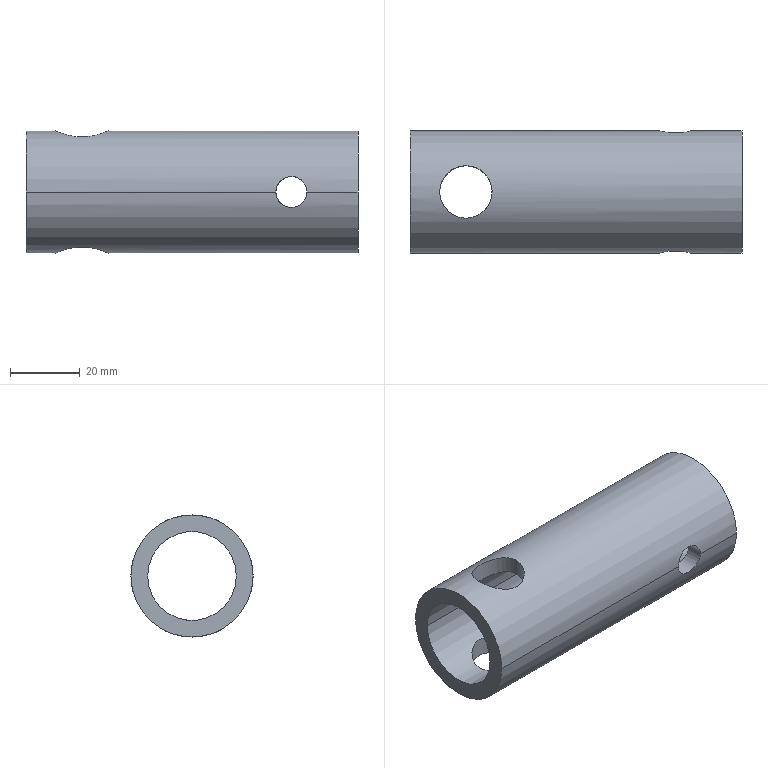Part | NX | features BREP 1 | 1 solid | 14 faces | box 94.996 x 34.925 x 34.925 mm | volume 40535 mm3 | cylinder 12 | plane 2 | commonest cylinder face diameters 8.89 x4 14.986 x4 25.4 x2 34.925 x2
STEP:
#1=CARTESIAN_POINT('',(-47.498,17.462,0.));
#2=VERTEX_POINT('',#1);
#3=CARTESIAN_POINT('',(-47.498,-17.462,0.));
#4=VERTEX_POINT('',#3);
#5=CARTESIAN_POINT('',(-47.498,0.,0.));
#6=DIRECTION('',(1.,0.,0.));
#7=DIRECTION('',(0.,1.,0.));
#8=AXIS2_PLACEMENT_3D('',#5,#6,#7);
#9=CIRCLE('',#8,17.462);
#10=EDGE_CURVE('',#2,#4,#9,.T.);
#11=ORIENTED_EDGE('',*,*,#10,.F.);
#12=CARTESIAN_POINT('',(-47.498,0.,0.));
#13=DIRECTION('',(1.,0.,0.));
#14=DIRECTION('',(0.,-1.,0.));
#15=AXIS2_PLACEMENT_3D('',#12,#13,#14);
#16=CIRCLE('',#15,17.462);
#17=EDGE_CURVE('',#4,#2,#16,.T.);
#18=ORIENTED_EDGE('',*,*,#17,.F.);
#19=EDGE_LOOP('',(#11,#18));
#20=FACE_BOUND('',#19,.T.);
#21=CARTESIAN_POINT('',(-47.498,12.7,0.));
#22=VERTEX_POINT('',#21);
#23=CARTESIAN_POINT('',(-47.498,-12.7,0.));
#24=VERTEX_POINT('',#23);
#25=CARTESIAN_POINT('',(-47.498,0.,0.));
#26=DIRECTION('',(-1.,0.,0.));
#27=DIRECTION('',(0.,1.,0.));
#28=AXIS2_PLACEMENT_3D('',#25,#26,#27);
#29=CIRCLE('',#28,12.7);
#30=EDGE_CURVE('',#22,#24,#29,.T.);
#31=ORIENTED_EDGE('',*,*,#30,.F.);
#32=CARTESIAN_POINT('',(-47.498,0.,0.));
#33=DIRECTION('',(-1.,0.,0.));
#34=DIRECTION('',(0.,-1.,0.));
#35=AXIS2_PLACEMENT_3D('',#32,#33,#34);
#36=CIRCLE('',#35,12.7);
#37=EDGE_CURVE('',#24,#22,#36,.T.);
#38=ORIENTED_EDGE('',*,*,#37,.F.);
#39=EDGE_LOOP('',(#31,#38));
#40=FACE_BOUND('',#39,.T.);
#41=CARTESIAN_POINT('',(-47.498,0.,0.));
#42=DIRECTION('',(1.,0.,0.));
#43=DIRECTION('',(0.,1.,0.));
#44=AXIS2_PLACEMENT_3D('',#41,#42,#43);
#45=PLANE('',#44);
#46=ADVANCED_FACE('',(#20,#40),#45,.F.);
#47=CARTESIAN_POINT('',(24.003,-17.462,0.));
#48=VERTEX_POINT('',#47);
#49=CARTESIAN_POINT('',(-47.498,-17.462,0.));
#50=DIRECTION('',(1.,0.,0.));
#51=VECTOR('',#50,1000.);
#52=LINE('',#49,#51);
#53=EDGE_CURVE('',#48,#4,#52,.F.);
#54=ORIENTED_EDGE('',*,*,#53,.T.);
#55=ORIENTED_EDGE('',*,*,#17,.T.);
#56=CARTESIAN_POINT('',(24.003,17.462,0.));
#57=VERTEX_POINT('',#56);
#58=CARTESIAN_POINT('',(-47.498,17.462,0.));
#59=DIRECTION('',(1.,0.,0.));
#60=VECTOR('',#59,1000.);
#61=LINE('',#58,#60);
#62=EDGE_CURVE('',#57,#2,#61,.F.);
#63=ORIENTED_EDGE('',*,*,#62,.F.);
#64=CARTESIAN_POINT('',(32.893,17.462,0.));
#65=VERTEX_POINT('',#64);
#66=CARTESIAN_POINT('',(24.003,17.462,0.));
#67=CARTESIAN_POINT('',(24.003,17.462,-1.164));
#68=CARTESIAN_POINT('',(24.94,17.187,-3.444));
#69=CARTESIAN_POINT('',(28.412,16.74,-4.935));
#70=CARTESIAN_POINT('',(31.928,17.178,-3.487));
#71=CARTESIAN_POINT('',(32.893,17.462,-1.178));
#72=CARTESIAN_POINT('',(32.893,17.462,0.));
#73=B_SPLINE_CURVE_WITH_KNOTS('',3,(#66,#67,#68,#69,#70,#71,#72),.UNSPECIFIED.,.F.,.F.,(4,1,1,1,4),(0.,0.25,0.5,0.75,1.),.UNSPECIFIED.);
#74=EDGE_CURVE('',#57,#65,#73,.T.);
#75=ORIENTED_EDGE('',*,*,#74,.T.);
#76=CARTESIAN_POINT('',(47.498,17.462,0.));
#77=VERTEX_POINT('',#76);
#78=CARTESIAN_POINT('',(32.893,17.462,0.));
#79=DIRECTION('',(1.,0.,0.));
#80=VECTOR('',#79,1000.);
#81=LINE('',#78,#80);
#82=EDGE_CURVE('',#65,#77,#81,.T.);
#83=ORIENTED_EDGE('',*,*,#82,.T.);
#84=CARTESIAN_POINT('',(47.498,-17.462,0.));
#85=VERTEX_POINT('',#84);
#86=CARTESIAN_POINT('',(47.498,0.,0.));
#87=DIRECTION('',(1.,0.,0.));
#88=DIRECTION('',(0.,-1.,0.));
#89=AXIS2_PLACEMENT_3D('',#86,#87,#88);
#90=CIRCLE('',#89,17.462);
#91=EDGE_CURVE('',#85,#77,#90,.T.);
#92=ORIENTED_EDGE('',*,*,#91,.F.);
#93=CARTESIAN_POINT('',(32.893,-17.462,0.));
#94=VERTEX_POINT('',#93);
#95=CARTESIAN_POINT('',(32.893,-17.462,0.));
#96=DIRECTION('',(1.,0.,0.));
#97=VECTOR('',#96,1000.);
#98=LINE('',#95,#97);
#99=EDGE_CURVE('',#94,#85,#98,.T.);
#100=ORIENTED_EDGE('',*,*,#99,.F.);
#101=CARTESIAN_POINT('',(32.893,-17.462,0.));
#102=CARTESIAN_POINT('',(32.893,-17.462,-1.177));
#103=CARTESIAN_POINT('',(31.929,-17.178,-3.484));
#104=CARTESIAN_POINT('',(28.419,-16.74,-4.934));
#105=CARTESIAN_POINT('',(24.943,-17.185,-3.449));
#106=CARTESIAN_POINT('',(24.003,-17.462,-1.165));
#107=CARTESIAN_POINT('',(24.003,-17.462,0.));
#108=B_SPLINE_CURVE_WITH_KNOTS('',3,(#101,#102,#103,#104,#105,#106,#107),.UNSPECIFIED.,.F.,.F.,(4,1,1,1,4),(0.,0.25,0.5,0.75,1.),.UNSPECIFIED.);
#109=EDGE_CURVE('',#94,#48,#108,.T.);
#110=ORIENTED_EDGE('',*,*,#109,.T.);
#111=EDGE_LOOP('',(#54,#55,#63,#75,#83,#92,#100,#110));
#112=FACE_BOUND('',#111,.T.);
#113=CARTESIAN_POINT('',(-38.989,0.,-17.462));
#114=VERTEX_POINT('',#113);
#115=CARTESIAN_POINT('',(-24.003,0.,-17.462));
#116=VERTEX_POINT('',#115);
#117=CARTESIAN_POINT('',(-38.989,0.,-17.462));
#118=CARTESIAN_POINT('',(-38.989,-2.022,-17.462));
#119=CARTESIAN_POINT('',(-37.692,-4.958,-16.852));
#120=CARTESIAN_POINT('',(-34.426,-7.1,-15.966));
#121=CARTESIAN_POINT('',(-31.48,-7.694,-15.675));
#122=CARTESIAN_POINT('',(-28.528,-7.083,-15.973));
#123=CARTESIAN_POINT('',(-25.304,-4.95,-16.853));
#124=CARTESIAN_POINT('',(-24.003,-2.022,-17.462));
#125=CARTESIAN_POINT('',(-24.003,0.,-17.462));
#126=B_SPLINE_CURVE_WITH_KNOTS('',3,(#117,#118,#119,#120,#121,#122,#123,#124,#125),.UNSPECIFIED.,.F.,.F.,(4,1,1,1,1,1,4),(0.,0.25,0.375,0.5,0.625,0.75,1.),.UNSPECIFIED.);
#127=EDGE_CURVE('',#114,#116,#126,.T.);
#128=ORIENTED_EDGE('',*,*,#127,.T.);
#129=CARTESIAN_POINT('',(-24.003,0.,-17.462));
#130=CARTESIAN_POINT('',(-24.003,2.019,-17.462));
#131=CARTESIAN_POINT('',(-25.295,4.952,-16.853));
#132=CARTESIAN_POINT('',(-28.564,7.1,-15.966));
#133=CARTESIAN_POINT('',(-31.512,7.694,-15.675));
#134=CARTESIAN_POINT('',(-34.465,7.083,-15.974));
#135=CARTESIAN_POINT('',(-37.693,4.945,-16.855));
#136=CARTESIAN_POINT('',(-38.989,2.019,-17.462));
#137=CARTESIAN_POINT('',(-38.989,0.,-17.462));
#138=B_SPLINE_CURVE_WITH_KNOTS('',3,(#129,#130,#131,#132,#133,#134,#135,#136,#137),.UNSPECIFIED.,.F.,.F.,(4,1,1,1,1,1,4),(0.,0.25,0.375,0.5,0.625,0.75,1.),.UNSPECIFIED.);
#139=EDGE_CURVE('',#116,#114,#138,.T.);
#140=ORIENTED_EDGE('',*,*,#139,.T.);
#141=EDGE_LOOP('',(#128,#140));
#142=FACE_BOUND('',#141,.T.);
#143=CARTESIAN_POINT('',(-47.498,0.,0.));
#144=DIRECTION('',(1.,0.,0.));
#145=DIRECTION('',(0.,-1.,0.));
#146=AXIS2_PLACEMENT_3D('',#143,#144,#145);
#147=CYLINDRICAL_SURFACE('',#146,17.462);
#148=ADVANCED_FACE('',(#112,#142),#147,.T.);
#149=CARTESIAN_POINT('',(32.893,-12.7,0.));
#150=VERTEX_POINT('',#149);
#151=CARTESIAN_POINT('',(32.893,-12.7,0.));
#152=DIRECTION('',(0.,-1.,0.));
#153=VECTOR('',#152,1000.);
#154=LINE('',#151,#153);
#155=EDGE_CURVE('',#94,#150,#154,.F.);
#156=ORIENTED_EDGE('',*,*,#155,.T.);
#157=CARTESIAN_POINT('',(24.003,-12.7,0.));
#158=VERTEX_POINT('',#157);
#159=CARTESIAN_POINT('',(32.893,-12.7,0.));
#160=CARTESIAN_POINT('',(32.893,-12.7,-0.278));
#161=CARTESIAN_POINT('',(32.848,-12.683,-0.8361));
#162=CARTESIAN_POINT('',(32.607,-12.602,-1.608));
#163=CARTESIAN_POINT('',(32.389,-12.532,-2.073));
#164=CARTESIAN_POINT('',(32.124,-12.451,-2.511));
#165=CARTESIAN_POINT('',(31.944,-12.399,-2.753));
#166=CARTESIAN_POINT('',(31.605,-12.306,-3.15));
#167=CARTESIAN_POINT('',(31.156,-12.2,-3.532));
#168=CARTESIAN_POINT('',(30.958,-12.157,-3.675));
#169=CARTESIAN_POINT('',(30.5,-12.07,-3.953));
#170=CARTESIAN_POINT('',(30.042,-11.999,-4.162));
#171=CARTESIAN_POINT('',(29.303,-11.916,-4.396));
#172=CARTESIAN_POINT('',(28.425,-11.886,-4.472));
#173=CARTESIAN_POINT('',(27.547,-11.919,-4.387));
#174=CARTESIAN_POINT('',(26.807,-12.005,-4.144));
#175=CARTESIAN_POINT('',(26.358,-12.077,-3.934));
#176=CARTESIAN_POINT('',(25.9,-12.165,-3.648));
#177=CARTESIAN_POINT('',(25.721,-12.204,-3.518));
#178=CARTESIAN_POINT('',(25.263,-12.313,-3.122));
#179=CARTESIAN_POINT('',(24.94,-12.403,-2.736));
#180=CARTESIAN_POINT('',(24.756,-12.456,-2.488));
#181=CARTESIAN_POINT('',(24.498,-12.535,-2.055));
#182=CARTESIAN_POINT('',(24.283,-12.604,-1.592));
#183=CARTESIAN_POINT('',(24.048,-12.683,-0.8289));
#184=CARTESIAN_POINT('',(24.003,-12.7,-0.2756));
#185=CARTESIAN_POINT('',(24.003,-12.7,0.));
#186=B_SPLINE_CURVE_WITH_KNOTS('',3,(#159,#160,#161,#162,#163,#164,#165,#166,#167,#168,#169,#170,#171,#172,#173,#174,#175,#176,#177,#178,#179,#180,#181,#182,#183,#184,#185),.UNSPECIFIED.,.F.,.F.,(4,1,1,1,1,1,1,1,1,1,1,1,1,1,1,1,1,1,1,1,1,1,1,1,4),(0.,0.0625,0.125,0.1562,0.1875,0.2188,0.25,0.2812,0.3125,0.3438,0.375,0.4375,0.5,0.5625,0.625,0.6562,0.6875,0.7188,0.75,0.7812,0.8125,0.8438,0.875,0.9375,1.),.UNSPECIFIED.);
#187=EDGE_CURVE('',#158,#150,#186,.F.);
#188=ORIENTED_EDGE('',*,*,#187,.F.);
#189=CARTESIAN_POINT('',(24.003,-12.7,0.));
#190=DIRECTION('',(0.,-1.,0.));
#191=VECTOR('',#190,1000.);
#192=LINE('',#189,#191);
#193=EDGE_CURVE('',#48,#158,#192,.F.);
#194=ORIENTED_EDGE('',*,*,#193,.F.);
#195=ORIENTED_EDGE('',*,*,#109,.F.);
#196=EDGE_LOOP('',(#156,#188,#194,#195));
#197=FACE_BOUND('',#196,.T.);
#198=CARTESIAN_POINT('',(28.448,22.86,0.));
#199=DIRECTION('',(0.,1.,0.));
#200=DIRECTION('',(1.,0.,0.));
#201=AXIS2_PLACEMENT_3D('',#198,#199,#200);
#202=CYLINDRICAL_SURFACE('',#201,4.445);
#203=ADVANCED_FACE('',(#197),#202,.F.);
#204=CARTESIAN_POINT('',(24.003,12.7,0.));
#205=VERTEX_POINT('',#204);
#206=CARTESIAN_POINT('',(24.003,17.462,0.));
#207=DIRECTION('',(0.,-1.,0.));
#208=VECTOR('',#207,1000.);
#209=LINE('',#206,#208);
#210=EDGE_CURVE('',#57,#205,#209,.T.);
#211=ORIENTED_EDGE('',*,*,#210,.T.);
#212=CARTESIAN_POINT('',(32.893,12.7,0.));
#213=VERTEX_POINT('',#212);
#214=CARTESIAN_POINT('',(24.003,12.7,0.));
#215=CARTESIAN_POINT('',(24.003,12.7,-0.2753));
#216=CARTESIAN_POINT('',(24.048,12.683,-0.828));
#217=CARTESIAN_POINT('',(24.283,12.604,-1.59));
#218=CARTESIAN_POINT('',(24.497,12.535,-2.053));
#219=CARTESIAN_POINT('',(24.755,12.456,-2.485));
#220=CARTESIAN_POINT('',(24.938,12.403,-2.734));
#221=CARTESIAN_POINT('',(25.259,12.314,-3.118));
#222=CARTESIAN_POINT('',(25.719,12.205,-3.516));
#223=CARTESIAN_POINT('',(25.894,12.166,-3.645));
#224=CARTESIAN_POINT('',(26.353,12.077,-3.931));
#225=CARTESIAN_POINT('',(26.801,12.006,-4.141));
#226=CARTESIAN_POINT('',(27.541,11.919,-4.386));
#227=CARTESIAN_POINT('',(28.42,11.886,-4.472));
#228=CARTESIAN_POINT('',(29.299,11.915,-4.397));
#229=CARTESIAN_POINT('',(30.038,11.998,-4.164));
#230=CARTESIAN_POINT('',(30.497,12.07,-3.955));
#231=CARTESIAN_POINT('',(30.955,12.156,-3.677));
#232=CARTESIAN_POINT('',(31.154,12.2,-3.533));
#233=CARTESIAN_POINT('',(31.603,12.305,-3.152));
#234=CARTESIAN_POINT('',(31.943,12.399,-2.754));
#235=CARTESIAN_POINT('',(32.123,12.451,-2.513));
#236=CARTESIAN_POINT('',(32.389,12.532,-2.074));
#237=CARTESIAN_POINT('',(32.606,12.602,-1.61));
#238=CARTESIAN_POINT('',(32.848,12.683,-0.8367));
#239=CARTESIAN_POINT('',(32.893,12.7,-0.2782));
#240=CARTESIAN_POINT('',(32.893,12.7,0.));
#241=B_SPLINE_CURVE_WITH_KNOTS('',3,(#214,#215,#216,#217,#218,#219,#220,#221,#222,#223,#224,#225,#226,#227,#228,#229,#230,#231,#232,#233,#234,#235,#236,#237,#238,#239,#240),.UNSPECIFIED.,.F.,.F.,(4,1,1,1,1,1,1,1,1,1,1,1,1,1,1,1,1,1,1,1,1,1,1,1,4),(0.,0.0625,0.125,0.1562,0.1875,0.2188,0.25,0.2812,0.3125,0.3438,0.375,0.4375,0.5,0.5625,0.625,0.6562,0.6875,0.7188,0.75,0.7812,0.8125,0.8438,0.875,0.9375,1.),.UNSPECIFIED.);
#242=EDGE_CURVE('',#213,#205,#241,.F.);
#243=ORIENTED_EDGE('',*,*,#242,.F.);
#244=CARTESIAN_POINT('',(32.893,17.462,0.));
#245=DIRECTION('',(0.,-1.,0.));
#246=VECTOR('',#245,1000.);
#247=LINE('',#244,#246);
#248=EDGE_CURVE('',#65,#213,#247,.T.);
#249=ORIENTED_EDGE('',*,*,#248,.F.);
#250=ORIENTED_EDGE('',*,*,#74,.F.);
#251=EDGE_LOOP('',(#211,#243,#249,#250));
#252=FACE_BOUND('',#251,.T.);
#253=CARTESIAN_POINT('',(28.448,22.86,0.));
#254=DIRECTION('',(0.,1.,0.));
#255=DIRECTION('',(1.,0.,0.));
#256=AXIS2_PLACEMENT_3D('',#253,#254,#255);
#257=CYLINDRICAL_SURFACE('',#256,4.445);
#258=ADVANCED_FACE('',(#252),#257,.F.);
#259=ORIENTED_EDGE('',*,*,#248,.T.);
#260=CARTESIAN_POINT('',(32.893,12.7,0.));
#261=CARTESIAN_POINT('',(32.893,12.7,0.2756));
#262=CARTESIAN_POINT('',(32.848,12.683,0.8289));
#263=CARTESIAN_POINT('',(32.613,12.604,1.592));
#264=CARTESIAN_POINT('',(32.398,12.535,2.055));
#265=CARTESIAN_POINT('',(32.14,12.456,2.488));
#266=CARTESIAN_POINT('',(31.956,12.403,2.736));
#267=CARTESIAN_POINT('',(31.633,12.313,3.122));
#268=CARTESIAN_POINT('',(31.174,12.204,3.518));
#269=CARTESIAN_POINT('',(30.997,12.165,3.648));
#270=CARTESIAN_POINT('',(30.537,12.077,3.934));
#271=CARTESIAN_POINT('',(30.089,12.006,4.144));
#272=CARTESIAN_POINT('',(29.349,11.919,4.387));
#273=CARTESIAN_POINT('',(28.471,11.886,4.472));
#274=CARTESIAN_POINT('',(27.593,11.916,4.396));
#275=CARTESIAN_POINT('',(26.855,11.999,4.163));
#276=CARTESIAN_POINT('',(26.396,12.07,3.953));
#277=CARTESIAN_POINT('',(25.938,12.157,3.675));
#278=CARTESIAN_POINT('',(25.74,12.2,3.532));
#279=CARTESIAN_POINT('',(25.291,12.306,3.15));
#280=CARTESIAN_POINT('',(24.952,12.399,2.753));
#281=CARTESIAN_POINT('',(24.772,12.451,2.511));
#282=CARTESIAN_POINT('',(24.507,12.532,2.073));
#283=CARTESIAN_POINT('',(24.289,12.602,1.608));
#284=CARTESIAN_POINT('',(24.048,12.683,0.8362));
#285=CARTESIAN_POINT('',(24.003,12.7,0.2781));
#286=CARTESIAN_POINT('',(24.003,12.7,0.));
#287=B_SPLINE_CURVE_WITH_KNOTS('',3,(#260,#261,#262,#263,#264,#265,#266,#267,#268,#269,#270,#271,#272,#273,#274,#275,#276,#277,#278,#279,#280,#281,#282,#283,#284,#285,#286),.UNSPECIFIED.,.F.,.F.,(4,1,1,1,1,1,1,1,1,1,1,1,1,1,1,1,1,1,1,1,1,1,1,1,4),(0.,0.0625,0.125,0.1562,0.1875,0.2188,0.25,0.2812,0.3125,0.3438,0.375,0.4375,0.5,0.5625,0.625,0.6562,0.6875,0.7188,0.75,0.7812,0.8125,0.8438,0.875,0.9375,1.),.UNSPECIFIED.);
#288=EDGE_CURVE('',#205,#213,#287,.F.);
#289=ORIENTED_EDGE('',*,*,#288,.F.);
#290=ORIENTED_EDGE('',*,*,#210,.F.);
#291=CARTESIAN_POINT('',(24.003,17.462,0.));
#292=CARTESIAN_POINT('',(24.003,17.462,0.2769));
#293=CARTESIAN_POINT('',(24.048,17.45,0.833));
#294=CARTESIAN_POINT('',(24.289,17.392,1.606));
#295=CARTESIAN_POINT('',(24.504,17.341,2.069));
#296=CARTESIAN_POINT('',(24.773,17.282,2.512));
#297=CARTESIAN_POINT('',(24.945,17.246,2.744));
#298=CARTESIAN_POINT('',(25.299,17.177,3.157));
#299=CARTESIAN_POINT('',(25.727,17.105,3.521));
#300=CARTESIAN_POINT('',(25.947,17.07,3.682));
#301=CARTESIAN_POINT('',(26.401,17.009,3.955));
#302=CARTESIAN_POINT('',(26.856,16.959,4.164));
#303=CARTESIAN_POINT('',(27.64,16.899,4.406));
#304=CARTESIAN_POINT('',(28.472,16.881,4.467));
#305=CARTESIAN_POINT('',(29.299,16.901,4.398));
#306=CARTESIAN_POINT('',(30.086,16.963,4.146));
#307=CARTESIAN_POINT('',(30.534,17.014,3.935));
#308=CARTESIAN_POINT('',(30.988,17.076,3.655));
#309=CARTESIAN_POINT('',(31.185,17.107,3.51));
#310=CARTESIAN_POINT('',(31.626,17.182,3.129));
#311=CARTESIAN_POINT('',(31.962,17.248,2.73));
#312=CARTESIAN_POINT('',(32.138,17.285,2.49));
#313=CARTESIAN_POINT('',(32.4,17.343,2.052));
#314=CARTESIAN_POINT('',(32.613,17.393,1.59));
#315=CARTESIAN_POINT('',(32.849,17.45,0.8261));
#316=CARTESIAN_POINT('',(32.893,17.462,0.2746));
#317=CARTESIAN_POINT('',(32.893,17.462,0.));
#318=B_SPLINE_CURVE_WITH_KNOTS('',3,(#291,#292,#293,#294,#295,#296,#297,#298,#299,#300,#301,#302,#303,#304,#305,#306,#307,#308,#309,#310,#311,#312,#313,#314,#315,#316,#317),.UNSPECIFIED.,.F.,.F.,(4,1,1,1,1,1,1,1,1,1,1,1,1,1,1,1,1,1,1,1,1,1,1,1,4),(0.,0.0625,0.125,0.1562,0.1875,0.2188,0.25,0.2812,0.3125,0.3438,0.375,0.4375,0.5,0.5625,0.625,0.6562,0.6875,0.7188,0.75,0.7812,0.8125,0.8438,0.875,0.9375,1.),.UNSPECIFIED.);
#319=EDGE_CURVE('',#65,#57,#318,.F.);
#320=ORIENTED_EDGE('',*,*,#319,.F.);
#321=EDGE_LOOP('',(#259,#289,#290,#320));
#322=FACE_BOUND('',#321,.T.);
#323=CARTESIAN_POINT('',(28.448,22.86,0.));
#324=DIRECTION('',(0.,1.,0.));
#325=DIRECTION('',(1.,0.,0.));
#326=AXIS2_PLACEMENT_3D('',#323,#324,#325);
#327=CYLINDRICAL_SURFACE('',#326,4.445);
#328=ADVANCED_FACE('',(#322),#327,.F.);
#329=ORIENTED_EDGE('',*,*,#193,.T.);
#330=CARTESIAN_POINT('',(24.003,-12.7,0.));
#331=CARTESIAN_POINT('',(24.003,-12.7,0.2782));
#332=CARTESIAN_POINT('',(24.048,-12.683,0.8366));
#333=CARTESIAN_POINT('',(24.29,-12.602,1.61));
#334=CARTESIAN_POINT('',(24.507,-12.532,2.074));
#335=CARTESIAN_POINT('',(24.773,-12.451,2.513));
#336=CARTESIAN_POINT('',(24.953,-12.399,2.754));
#337=CARTESIAN_POINT('',(25.293,-12.305,3.152));
#338=CARTESIAN_POINT('',(25.742,-12.2,3.533));
#339=CARTESIAN_POINT('',(25.941,-12.156,3.677));
#340=CARTESIAN_POINT('',(26.399,-12.07,3.955));
#341=CARTESIAN_POINT('',(26.858,-11.998,4.164));
#342=CARTESIAN_POINT('',(27.597,-11.915,4.397));
#343=CARTESIAN_POINT('',(28.476,-11.886,4.472));
#344=CARTESIAN_POINT('',(29.355,-11.919,4.386));
#345=CARTESIAN_POINT('',(30.095,-12.006,4.141));
#346=CARTESIAN_POINT('',(30.543,-12.077,3.931));
#347=CARTESIAN_POINT('',(31.002,-12.166,3.645));
#348=CARTESIAN_POINT('',(31.177,-12.205,3.516));
#349=CARTESIAN_POINT('',(31.637,-12.314,3.118));
#350=CARTESIAN_POINT('',(31.958,-12.403,2.734));
#351=CARTESIAN_POINT('',(32.142,-12.456,2.485));
#352=CARTESIAN_POINT('',(32.399,-12.535,2.053));
#353=CARTESIAN_POINT('',(32.613,-12.604,1.59));
#354=CARTESIAN_POINT('',(32.848,-12.683,0.8281));
#355=CARTESIAN_POINT('',(32.893,-12.7,0.2753));
#356=CARTESIAN_POINT('',(32.893,-12.7,0.));
#357=B_SPLINE_CURVE_WITH_KNOTS('',3,(#330,#331,#332,#333,#334,#335,#336,#337,#338,#339,#340,#341,#342,#343,#344,#345,#346,#347,#348,#349,#350,#351,#352,#353,#354,#355,#356),.UNSPECIFIED.,.F.,.F.,(4,1,1,1,1,1,1,1,1,1,1,1,1,1,1,1,1,1,1,1,1,1,1,1,4),(0.,0.0625,0.125,0.1562,0.1875,0.2188,0.25,0.2812,0.3125,0.3438,0.375,0.4375,0.5,0.5625,0.625,0.6562,0.6875,0.7188,0.75,0.7812,0.8125,0.8438,0.875,0.9375,1.),.UNSPECIFIED.);
#358=EDGE_CURVE('',#150,#158,#357,.F.);
#359=ORIENTED_EDGE('',*,*,#358,.F.);
#360=ORIENTED_EDGE('',*,*,#155,.F.);
#361=CARTESIAN_POINT('',(32.893,-17.462,0.));
#362=CARTESIAN_POINT('',(32.893,-17.462,0.2743));
#363=CARTESIAN_POINT('',(32.849,-17.45,0.8252));
#364=CARTESIAN_POINT('',(32.614,-17.393,1.588));
#365=CARTESIAN_POINT('',(32.401,-17.343,2.05));
#366=CARTESIAN_POINT('',(32.14,-17.286,2.487));
#367=CARTESIAN_POINT('',(31.964,-17.249,2.727));
#368=CARTESIAN_POINT('',(31.63,-17.183,3.125));
#369=CARTESIAN_POINT('',(31.188,-17.107,3.508));
#370=CARTESIAN_POINT('',(30.993,-17.077,3.651));
#371=CARTESIAN_POINT('',(30.539,-17.015,3.932));
#372=CARTESIAN_POINT('',(30.093,-16.964,4.143));
#373=CARTESIAN_POINT('',(29.304,-16.901,4.397));
#374=CARTESIAN_POINT('',(28.478,-16.881,4.467));
#375=CARTESIAN_POINT('',(27.644,-16.899,4.406));
#376=CARTESIAN_POINT('',(26.861,-16.959,4.166));
#377=CARTESIAN_POINT('',(26.402,-17.009,3.956));
#378=CARTESIAN_POINT('',(25.949,-17.07,3.683));
#379=CARTESIAN_POINT('',(25.733,-17.104,3.527));
#380=CARTESIAN_POINT('',(25.299,-17.176,3.158));
#381=CARTESIAN_POINT('',(24.946,-17.246,2.746));
#382=CARTESIAN_POINT('',(24.775,-17.282,2.514));
#383=CARTESIAN_POINT('',(24.505,-17.341,2.07));
#384=CARTESIAN_POINT('',(24.289,-17.392,1.607));
#385=CARTESIAN_POINT('',(24.048,-17.45,0.8336));
#386=CARTESIAN_POINT('',(24.003,-17.462,0.2771));
#387=CARTESIAN_POINT('',(24.003,-17.462,0.));
#388=B_SPLINE_CURVE_WITH_KNOTS('',3,(#361,#362,#363,#364,#365,#366,#367,#368,#369,#370,#371,#372,#373,#374,#375,#376,#377,#378,#379,#380,#381,#382,#383,#384,#385,#386,#387),.UNSPECIFIED.,.F.,.F.,(4,1,1,1,1,1,1,1,1,1,1,1,1,1,1,1,1,1,1,1,1,1,1,1,4),(0.,0.0625,0.125,0.1562,0.1875,0.2188,0.25,0.2812,0.3125,0.3438,0.375,0.4375,0.5,0.5625,0.625,0.6562,0.6875,0.7188,0.75,0.7812,0.8125,0.8438,0.875,0.9375,1.),.UNSPECIFIED.);
#389=EDGE_CURVE('',#48,#94,#388,.F.);
#390=ORIENTED_EDGE('',*,*,#389,.F.);
#391=EDGE_LOOP('',(#329,#359,#360,#390));
#392=FACE_BOUND('',#391,.T.);
#393=CARTESIAN_POINT('',(28.448,22.86,0.));
#394=DIRECTION('',(0.,1.,0.));
#395=DIRECTION('',(1.,0.,0.));
#396=AXIS2_PLACEMENT_3D('',#393,#394,#395);
#397=CYLINDRICAL_SURFACE('',#396,4.445);
#398=ADVANCED_FACE('',(#392),#397,.F.);
#399=ORIENTED_EDGE('',*,*,#62,.T.);
#400=ORIENTED_EDGE('',*,*,#10,.T.);
#401=ORIENTED_EDGE('',*,*,#53,.F.);
#402=ORIENTED_EDGE('',*,*,#389,.T.);
#403=ORIENTED_EDGE('',*,*,#99,.T.);
#404=CARTESIAN_POINT('',(47.498,0.,0.));
#405=DIRECTION('',(1.,0.,0.));
#406=DIRECTION('',(0.,1.,0.));
#407=AXIS2_PLACEMENT_3D('',#404,#405,#406);
#408=CIRCLE('',#407,17.462);
#409=EDGE_CURVE('',#77,#85,#408,.T.);
#410=ORIENTED_EDGE('',*,*,#409,.F.);
#411=ORIENTED_EDGE('',*,*,#82,.F.);
#412=ORIENTED_EDGE('',*,*,#319,.T.);
#413=EDGE_LOOP('',(#399,#400,#401,#402,#403,#410,#411,#412));
#414=FACE_BOUND('',#413,.T.);
#415=CARTESIAN_POINT('',(-24.003,0.,17.462));
#416=VERTEX_POINT('',#415);
#417=CARTESIAN_POINT('',(-38.989,0.,17.462));
#418=VERTEX_POINT('',#417);
#419=CARTESIAN_POINT('',(-24.003,0.,17.462));
#420=CARTESIAN_POINT('',(-24.003,-2.019,17.462));
#421=CARTESIAN_POINT('',(-25.299,-4.945,16.855));
#422=CARTESIAN_POINT('',(-28.527,-7.083,15.974));
#423=CARTESIAN_POINT('',(-31.48,-7.694,15.675));
#424=CARTESIAN_POINT('',(-34.428,-7.1,15.966));
#425=CARTESIAN_POINT('',(-37.697,-4.952,16.853));
#426=CARTESIAN_POINT('',(-38.989,-2.02,17.462));
#427=CARTESIAN_POINT('',(-38.989,0.,17.462));
#428=B_SPLINE_CURVE_WITH_KNOTS('',3,(#419,#420,#421,#422,#423,#424,#425,#426,#427),.UNSPECIFIED.,.F.,.F.,(4,1,1,1,1,1,4),(0.,0.25,0.375,0.5,0.625,0.75,1.),.UNSPECIFIED.);
#429=EDGE_CURVE('',#416,#418,#428,.T.);
#430=ORIENTED_EDGE('',*,*,#429,.T.);
#431=CARTESIAN_POINT('',(-38.989,0.,17.462));
#432=CARTESIAN_POINT('',(-38.989,2.021,17.462));
#433=CARTESIAN_POINT('',(-37.688,4.95,16.853));
#434=CARTESIAN_POINT('',(-34.464,7.083,15.973));
#435=CARTESIAN_POINT('',(-31.512,7.694,15.675));
#436=CARTESIAN_POINT('',(-28.566,7.1,15.966));
#437=CARTESIAN_POINT('',(-25.3,4.957,16.852));
#438=CARTESIAN_POINT('',(-24.003,2.022,17.462));
#439=CARTESIAN_POINT('',(-24.003,0.,17.462));
#440=B_SPLINE_CURVE_WITH_KNOTS('',3,(#431,#432,#433,#434,#435,#436,#437,#438,#439),.UNSPECIFIED.,.F.,.F.,(4,1,1,1,1,1,4),(0.,0.25,0.375,0.5,0.625,0.75,1.),.UNSPECIFIED.);
#441=EDGE_CURVE('',#418,#416,#440,.T.);
#442=ORIENTED_EDGE('',*,*,#441,.T.);
#443=EDGE_LOOP('',(#430,#442));
#444=FACE_BOUND('',#443,.T.);
#445=CARTESIAN_POINT('',(-47.498,0.,0.));
#446=DIRECTION('',(1.,0.,0.));
#447=DIRECTION('',(0.,-1.,0.));
#448=AXIS2_PLACEMENT_3D('',#445,#446,#447);
#449=CYLINDRICAL_SURFACE('',#448,17.462);
#450=ADVANCED_FACE('',(#414,#444),#449,.T.);
#451=ORIENTED_EDGE('',*,*,#409,.T.);
#452=ORIENTED_EDGE('',*,*,#91,.T.);
#453=EDGE_LOOP('',(#451,#452));
#454=FACE_BOUND('',#453,.T.);
#455=CARTESIAN_POINT('',(47.498,12.7,0.));
#456=VERTEX_POINT('',#455);
#457=CARTESIAN_POINT('',(47.498,-12.7,0.));
#458=VERTEX_POINT('',#457);
#459=CARTESIAN_POINT('',(47.498,0.,0.));
#460=DIRECTION('',(-1.,0.,0.));
#461=DIRECTION('',(0.,1.,0.));
#462=AXIS2_PLACEMENT_3D('',#459,#460,#461);
#463=CIRCLE('',#462,12.7);
#464=EDGE_CURVE('',#456,#458,#463,.T.);
#465=ORIENTED_EDGE('',*,*,#464,.T.);
#466=CARTESIAN_POINT('',(47.498,0.,0.));
#467=DIRECTION('',(-1.,0.,0.));
#468=DIRECTION('',(0.,-1.,0.));
#469=AXIS2_PLACEMENT_3D('',#466,#467,#468);
#470=CIRCLE('',#469,12.7);
#471=EDGE_CURVE('',#458,#456,#470,.T.);
#472=ORIENTED_EDGE('',*,*,#471,.T.);
#473=EDGE_LOOP('',(#465,#472));
#474=FACE_BOUND('',#473,.T.);
#475=CARTESIAN_POINT('',(47.498,0.,0.));
#476=DIRECTION('',(1.,0.,0.));
#477=DIRECTION('',(0.,1.,0.));
#478=AXIS2_PLACEMENT_3D('',#475,#476,#477);
#479=PLANE('',#478);
#480=ADVANCED_FACE('',(#454,#474),#479,.T.);
#481=CARTESIAN_POINT('',(32.893,12.7,0.));
#482=DIRECTION('',(1.,0.,0.));
#483=VECTOR('',#482,1000.);
#484=LINE('',#481,#483);
#485=EDGE_CURVE('',#456,#213,#484,.F.);
#486=ORIENTED_EDGE('',*,*,#485,.F.);
#487=ORIENTED_EDGE('',*,*,#471,.F.);
#488=CARTESIAN_POINT('',(32.893,-12.7,0.));
#489=DIRECTION('',(1.,0.,0.));
#490=VECTOR('',#489,1000.);
#491=LINE('',#488,#490);
#492=EDGE_CURVE('',#458,#150,#491,.F.);
#493=ORIENTED_EDGE('',*,*,#492,.T.);
#494=ORIENTED_EDGE('',*,*,#358,.T.);
#495=CARTESIAN_POINT('',(-47.498,-12.7,0.));
#496=DIRECTION('',(1.,0.,0.));
#497=VECTOR('',#496,1000.);
#498=LINE('',#495,#497);
#499=EDGE_CURVE('',#24,#158,#498,.T.);
#500=ORIENTED_EDGE('',*,*,#499,.F.);
#501=ORIENTED_EDGE('',*,*,#37,.T.);
#502=CARTESIAN_POINT('',(-47.498,12.7,0.));
#503=DIRECTION('',(1.,0.,0.));
#504=VECTOR('',#503,1000.);
#505=LINE('',#502,#504);
#506=EDGE_CURVE('',#22,#205,#505,.T.);
#507=ORIENTED_EDGE('',*,*,#506,.T.);
#508=ORIENTED_EDGE('',*,*,#288,.T.);
#509=EDGE_LOOP('',(#486,#487,#493,#494,#500,#501,#507,#508));
#510=FACE_BOUND('',#509,.T.);
#511=CARTESIAN_POINT('',(-38.989,0.,12.7));
#512=VERTEX_POINT('',#511);
#513=CARTESIAN_POINT('',(-24.003,0.,12.7));
#514=VERTEX_POINT('',#513);
#515=CARTESIAN_POINT('',(-38.989,0.,12.7));
#516=CARTESIAN_POINT('',(-38.989,-0.9667,12.7));
#517=CARTESIAN_POINT('',(-38.649,-2.834,12.494));
#518=CARTESIAN_POINT('',(-36.884,-5.531,11.525));
#519=CARTESIAN_POINT('',(-34.234,-7.175,10.5));
#520=CARTESIAN_POINT('',(-31.501,-7.651,10.131));
#521=CARTESIAN_POINT('',(-28.769,-7.179,10.497));
#522=CARTESIAN_POINT('',(-26.116,-5.538,11.521));
#523=CARTESIAN_POINT('',(-24.349,-2.849,12.49));
#524=CARTESIAN_POINT('',(-24.003,-0.9711,12.7));
#525=CARTESIAN_POINT('',(-24.003,0.,12.7));
#526=B_SPLINE_CURVE_WITH_KNOTS('',3,(#515,#516,#517,#518,#519,#520,#521,#522,#523,#524,#525),.UNSPECIFIED.,.F.,.F.,(4,1,1,1,1,1,1,1,4),(0.,0.125,0.25,0.375,0.5,0.625,0.75,0.875,1.),.UNSPECIFIED.);
#527=EDGE_CURVE('',#512,#514,#526,.T.);
#528=ORIENTED_EDGE('',*,*,#527,.T.);
#529=CARTESIAN_POINT('',(-24.003,0.,12.7));
#530=CARTESIAN_POINT('',(-24.003,0.9666,12.7));
#531=CARTESIAN_POINT('',(-24.343,2.833,12.494));
#532=CARTESIAN_POINT('',(-26.108,5.532,11.525));
#533=CARTESIAN_POINT('',(-28.758,7.175,10.5));
#534=CARTESIAN_POINT('',(-31.491,7.651,10.131));
#535=CARTESIAN_POINT('',(-34.223,7.179,10.497));
#536=CARTESIAN_POINT('',(-36.875,5.539,11.52));
#537=CARTESIAN_POINT('',(-38.643,2.849,12.49));
#538=CARTESIAN_POINT('',(-38.989,0.9711,12.7));
#539=CARTESIAN_POINT('',(-38.989,0.,12.7));
#540=B_SPLINE_CURVE_WITH_KNOTS('',3,(#529,#530,#531,#532,#533,#534,#535,#536,#537,#538,#539),.UNSPECIFIED.,.F.,.F.,(4,1,1,1,1,1,1,1,4),(0.,0.125,0.25,0.375,0.5,0.625,0.75,0.875,1.),.UNSPECIFIED.);
#541=EDGE_CURVE('',#514,#512,#540,.T.);
#542=ORIENTED_EDGE('',*,*,#541,.T.);
#543=EDGE_LOOP('',(#528,#542));
#544=FACE_BOUND('',#543,.T.);
#545=CARTESIAN_POINT('',(-47.498,0.,0.));
#546=DIRECTION('',(1.,0.,0.));
#547=DIRECTION('',(0.,-1.,0.));
#548=AXIS2_PLACEMENT_3D('',#545,#546,#547);
#549=CYLINDRICAL_SURFACE('',#548,12.7);
#550=ADVANCED_FACE('',(#510,#544),#549,.F.);
#551=ORIENTED_EDGE('',*,*,#492,.F.);
#552=ORIENTED_EDGE('',*,*,#464,.F.);
#553=ORIENTED_EDGE('',*,*,#485,.T.);
#554=ORIENTED_EDGE('',*,*,#242,.T.);
#555=ORIENTED_EDGE('',*,*,#506,.F.);
#556=ORIENTED_EDGE('',*,*,#30,.T.);
#557=ORIENTED_EDGE('',*,*,#499,.T.);
#558=ORIENTED_EDGE('',*,*,#187,.T.);
#559=EDGE_LOOP('',(#551,#552,#553,#554,#555,#556,#557,#558));
#560=FACE_BOUND('',#559,.T.);
#561=CARTESIAN_POINT('',(-24.003,0.,-12.7));
#562=VERTEX_POINT('',#561);
#563=CARTESIAN_POINT('',(-38.989,0.,-12.7));
#564=VERTEX_POINT('',#563);
#565=CARTESIAN_POINT('',(-24.003,0.,-12.7));
#566=CARTESIAN_POINT('',(-24.003,-0.9709,-12.7));
#567=CARTESIAN_POINT('',(-24.349,-2.849,-12.49));
#568=CARTESIAN_POINT('',(-26.117,-5.539,-11.52));
#569=CARTESIAN_POINT('',(-28.769,-7.179,-10.497));
#570=CARTESIAN_POINT('',(-31.501,-7.651,-10.131));
#571=CARTESIAN_POINT('',(-34.234,-7.175,-10.5));
#572=CARTESIAN_POINT('',(-36.884,-5.532,-11.525));
#573=CARTESIAN_POINT('',(-38.649,-2.833,-12.494));
#574=CARTESIAN_POINT('',(-38.989,-0.9668,-12.7));
#575=CARTESIAN_POINT('',(-38.989,0.,-12.7));
#576=B_SPLINE_CURVE_WITH_KNOTS('',3,(#565,#566,#567,#568,#569,#570,#571,#572,#573,#574,#575),.UNSPECIFIED.,.F.,.F.,(4,1,1,1,1,1,1,1,4),(0.,0.125,0.25,0.375,0.5,0.625,0.75,0.875,1.),.UNSPECIFIED.);
#577=EDGE_CURVE('',#562,#564,#576,.T.);
#578=ORIENTED_EDGE('',*,*,#577,.T.);
#579=CARTESIAN_POINT('',(-38.989,0.,-12.7));
#580=CARTESIAN_POINT('',(-38.989,0.9709,-12.7));
#581=CARTESIAN_POINT('',(-38.643,2.849,-12.49));
#582=CARTESIAN_POINT('',(-36.876,5.538,-11.521));
#583=CARTESIAN_POINT('',(-34.223,7.179,-10.497));
#584=CARTESIAN_POINT('',(-31.491,7.651,-10.131));
#585=CARTESIAN_POINT('',(-28.758,7.175,-10.5));
#586=CARTESIAN_POINT('',(-26.108,5.531,-11.525));
#587=CARTESIAN_POINT('',(-24.343,2.834,-12.494));
#588=CARTESIAN_POINT('',(-24.003,0.9668,-12.7));
#589=CARTESIAN_POINT('',(-24.003,0.,-12.7));
#590=B_SPLINE_CURVE_WITH_KNOTS('',3,(#579,#580,#581,#582,#583,#584,#585,#586,#587,#588,#589),.UNSPECIFIED.,.F.,.F.,(4,1,1,1,1,1,1,1,4),(0.,0.125,0.25,0.375,0.5,0.625,0.75,0.875,1.),.UNSPECIFIED.);
#591=EDGE_CURVE('',#564,#562,#590,.T.);
#592=ORIENTED_EDGE('',*,*,#591,.T.);
#593=EDGE_LOOP('',(#578,#592));
#594=FACE_BOUND('',#593,.T.);
#595=CARTESIAN_POINT('',(-47.498,0.,0.));
#596=DIRECTION('',(1.,0.,0.));
#597=DIRECTION('',(0.,-1.,0.));
#598=AXIS2_PLACEMENT_3D('',#595,#596,#597);
#599=CYLINDRICAL_SURFACE('',#598,12.7);
#600=ADVANCED_FACE('',(#560,#594),#599,.F.);
#601=CARTESIAN_POINT('',(-24.003,0.,-12.7));
#602=DIRECTION('',(0.,0.,-1.));
#603=VECTOR('',#602,1000.);
#604=LINE('',#601,#603);
#605=EDGE_CURVE('',#116,#562,#604,.F.);
#606=ORIENTED_EDGE('',*,*,#605,.T.);
#607=ORIENTED_EDGE('',*,*,#591,.F.);
#608=CARTESIAN_POINT('',(-38.989,0.,-12.7));
#609=DIRECTION('',(0.,0.,-1.));
#610=VECTOR('',#609,1000.);
#611=LINE('',#608,#610);
#612=EDGE_CURVE('',#114,#564,#611,.F.);
#613=ORIENTED_EDGE('',*,*,#612,.F.);
#614=ORIENTED_EDGE('',*,*,#139,.F.);
#615=EDGE_LOOP('',(#606,#607,#613,#614));
#616=FACE_BOUND('',#615,.T.);
#617=CARTESIAN_POINT('',(-31.496,0.,22.86));
#618=DIRECTION('',(0.,0.,1.));
#619=DIRECTION('',(1.,0.,0.));
#620=AXIS2_PLACEMENT_3D('',#617,#618,#619);
#621=CYLINDRICAL_SURFACE('',#620,7.493);
#622=ADVANCED_FACE('',(#616),#621,.F.);
#623=CARTESIAN_POINT('',(-38.989,0.,17.462));
#624=DIRECTION('',(0.,0.,-1.));
#625=VECTOR('',#624,1000.);
#626=LINE('',#623,#625);
#627=EDGE_CURVE('',#418,#512,#626,.T.);
#628=ORIENTED_EDGE('',*,*,#627,.T.);
#629=ORIENTED_EDGE('',*,*,#541,.F.);
#630=CARTESIAN_POINT('',(-24.003,0.,17.462));
#631=DIRECTION('',(0.,0.,-1.));
#632=VECTOR('',#631,1000.);
#633=LINE('',#630,#632);
#634=EDGE_CURVE('',#416,#514,#633,.T.);
#635=ORIENTED_EDGE('',*,*,#634,.F.);
#636=ORIENTED_EDGE('',*,*,#441,.F.);
#637=EDGE_LOOP('',(#628,#629,#635,#636));
#638=FACE_BOUND('',#637,.T.);
#639=CARTESIAN_POINT('',(-31.496,0.,22.86));
#640=DIRECTION('',(0.,0.,1.));
#641=DIRECTION('',(1.,0.,0.));
#642=AXIS2_PLACEMENT_3D('',#639,#640,#641);
#643=CYLINDRICAL_SURFACE('',#642,7.493);
#644=ADVANCED_FACE('',(#638),#643,.F.);
#645=ORIENTED_EDGE('',*,*,#612,.T.);
#646=ORIENTED_EDGE('',*,*,#577,.F.);
#647=ORIENTED_EDGE('',*,*,#605,.F.);
#648=ORIENTED_EDGE('',*,*,#127,.F.);
#649=EDGE_LOOP('',(#645,#646,#647,#648));
#650=FACE_BOUND('',#649,.T.);
#651=CARTESIAN_POINT('',(-31.496,0.,22.86));
#652=DIRECTION('',(0.,0.,1.));
#653=DIRECTION('',(1.,0.,0.));
#654=AXIS2_PLACEMENT_3D('',#651,#652,#653);
#655=CYLINDRICAL_SURFACE('',#654,7.493);
#656=ADVANCED_FACE('',(#650),#655,.F.);
#657=ORIENTED_EDGE('',*,*,#634,.T.);
#658=ORIENTED_EDGE('',*,*,#527,.F.);
#659=ORIENTED_EDGE('',*,*,#627,.F.);
#660=ORIENTED_EDGE('',*,*,#429,.F.);
#661=EDGE_LOOP('',(#657,#658,#659,#660));
#662=FACE_BOUND('',#661,.T.);
#663=CARTESIAN_POINT('',(-31.496,0.,22.86));
#664=DIRECTION('',(0.,0.,1.));
#665=DIRECTION('',(1.,0.,0.));
#666=AXIS2_PLACEMENT_3D('',#663,#664,#665);
#667=CYLINDRICAL_SURFACE('',#666,7.493);
#668=ADVANCED_FACE('',(#662),#667,.F.);
#669=CLOSED_SHELL('',(#46,#148,#203,#258,#328,#398,#450,#480,#550,#600,#622,#644,#656,#668));
#670=MANIFOLD_SOLID_BREP('',#669);
#671=(LENGTH_UNIT()NAMED_UNIT(*)SI_UNIT(.MILLI.,.METRE.));
#672=UNCERTAINTY_MEASURE_WITH_UNIT(LENGTH_MEASURE(0.0508),#671,'','');
#673=(NAMED_UNIT(*)PLANE_ANGLE_UNIT()SI_UNIT($,.RADIAN.));
#674=(NAMED_UNIT(*)SI_UNIT($,.STERADIAN.)SOLID_ANGLE_UNIT());
#675=(GEOMETRIC_REPRESENTATION_CONTEXT(3)GLOBAL_UNCERTAINTY_ASSIGNED_CONTEXT((#672))GLOBAL_UNIT_ASSIGNED_CONTEXT((#671,#673,#674))REPRESENTATION_CONTEXT('',''));
#676=ADVANCED_BREP_SHAPE_REPRESENTATION('',(#670),#675);